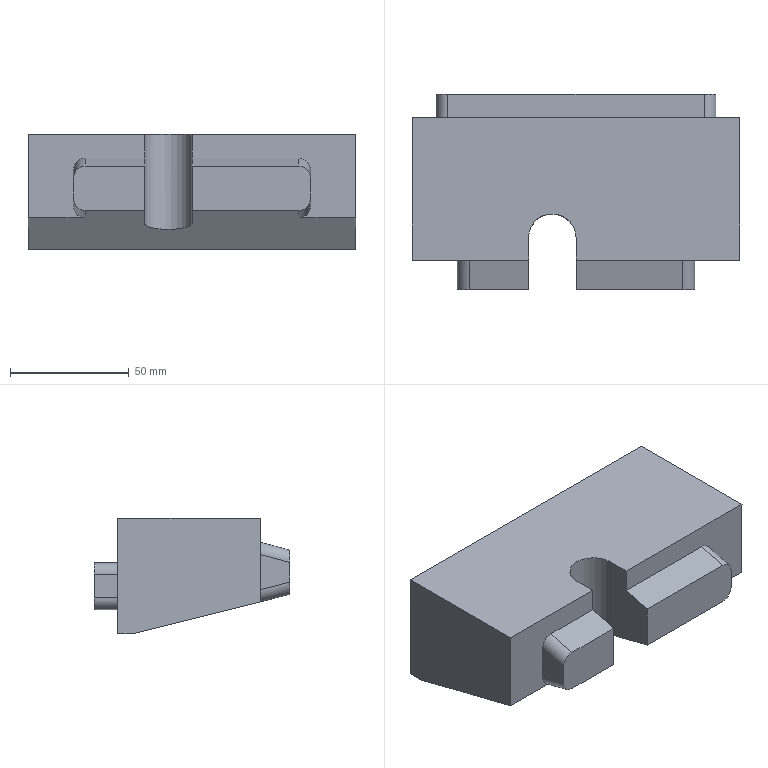Part | STEP file | WEDGE-2_id574_x_t | 1 solid | 30 faces | box 138 x 82.5 x 48.5 mm | volume 384224 mm3 | plane 21 | cylinder 9 | commonest cylinder face diameters 10 x8 20 x1
STEP:
#1=CARTESIAN_POINT('',(-79.,10.5,241.503));
#2=VERTEX_POINT('',#1);
#3=CARTESIAN_POINT('',(-79.,10.5,251.503));
#4=VERTEX_POINT('',#3);
#5=CARTESIAN_POINT('',(-79.,10.5,232.37));
#6=DIRECTION('',(0.,0.,1.));
#7=VECTOR('',#6,1.);
#8=LINE('',#5,#7);
#9=EDGE_CURVE('',#2,#4,#8,.T.);
#10=ORIENTED_EDGE('',*,*,#9,.T.);
#11=CARTESIAN_POINT('',(-74.,10.5,256.503));
#12=VERTEX_POINT('',#11);
#13=CARTESIAN_POINT('',(-74.,10.5,251.503));
#14=DIRECTION('',(0.,-1.,0.));
#15=DIRECTION('',(0.,0.,-1.));
#16=AXIS2_PLACEMENT_3D('',#13,#14,#15);
#17=CIRCLE('',#16,5.);
#18=EDGE_CURVE('',#12,#4,#17,.T.);
#19=ORIENTED_EDGE('',*,*,#18,.F.);
#20=CARTESIAN_POINT('',(34.,10.5,256.503));
#21=VERTEX_POINT('',#20);
#22=CARTESIAN_POINT('',(-89.,10.5,256.503));
#23=DIRECTION('',(-1.,0.,0.));
#24=VECTOR('',#23,1.);
#25=LINE('',#22,#24);
#26=EDGE_CURVE('',#21,#12,#25,.T.);
#27=ORIENTED_EDGE('',*,*,#26,.F.);
#28=CARTESIAN_POINT('',(39.,10.5,251.503));
#29=VERTEX_POINT('',#28);
#30=CARTESIAN_POINT('',(34.,10.5,251.503));
#31=DIRECTION('',(0.,-1.,0.));
#32=DIRECTION('',(0.,0.,1.));
#33=AXIS2_PLACEMENT_3D('',#30,#31,#32);
#34=CIRCLE('',#33,5.);
#35=EDGE_CURVE('',#29,#21,#34,.T.);
#36=ORIENTED_EDGE('',*,*,#35,.F.);
#37=CARTESIAN_POINT('',(39.,10.5,241.503));
#38=VERTEX_POINT('',#37);
#39=CARTESIAN_POINT('',(39.,10.5,260.794));
#40=DIRECTION('',(0.,0.,-1.));
#41=VECTOR('',#40,1.);
#42=LINE('',#39,#41);
#43=EDGE_CURVE('',#29,#38,#42,.T.);
#44=ORIENTED_EDGE('',*,*,#43,.T.);
#45=CARTESIAN_POINT('',(34.,10.5,236.503));
#46=VERTEX_POINT('',#45);
#47=CARTESIAN_POINT('',(34.,10.5,241.503));
#48=DIRECTION('',(0.,-1.,0.));
#49=DIRECTION('',(0.,0.,-1.));
#50=AXIS2_PLACEMENT_3D('',#47,#48,#49);
#51=CIRCLE('',#50,5.);
#52=EDGE_CURVE('',#46,#38,#51,.T.);
#53=ORIENTED_EDGE('',*,*,#52,.F.);
#54=CARTESIAN_POINT('',(-74.,10.5,236.503));
#55=VERTEX_POINT('',#54);
#56=CARTESIAN_POINT('',(-89.,10.5,236.503));
#57=DIRECTION('',(1.,0.,0.));
#58=VECTOR('',#57,1.);
#59=LINE('',#56,#58);
#60=EDGE_CURVE('',#55,#46,#59,.T.);
#61=ORIENTED_EDGE('',*,*,#60,.F.);
#62=CARTESIAN_POINT('',(-74.,10.5,241.503));
#63=DIRECTION('',(0.,-1.,0.));
#64=DIRECTION('',(0.,0.,1.));
#65=AXIS2_PLACEMENT_3D('',#62,#63,#64);
#66=CIRCLE('',#65,5.);
#67=EDGE_CURVE('',#2,#55,#66,.T.);
#68=ORIENTED_EDGE('',*,*,#67,.F.);
#69=EDGE_LOOP('',(#10,#19,#27,#36,#44,#53,#61,#68));
#70=FACE_OUTER_BOUND('',#69,.T.);
#71=CARTESIAN_POINT('',(-89.,10.5,236.503));
#72=DIRECTION('',(0.,1.,0.));
#73=DIRECTION('',(0.,0.,1.));
#74=AXIS2_PLACEMENT_3D('',#71,#72,#73);
#75=PLANE('',#74);
#76=ADVANCED_FACE('',(#70),#75,.T.);
#77=ORIENTED_EDGE('',*,*,#18,.T.);
#78=CARTESIAN_POINT('',(-79.,0.5,251.503));
#79=VERTEX_POINT('',#78);
#80=CARTESIAN_POINT('',(-79.,0.5,251.503));
#81=DIRECTION('',(0.,-1.,0.));
#82=VECTOR('',#81,1.);
#83=LINE('',#80,#82);
#84=EDGE_CURVE('',#4,#79,#83,.T.);
#85=ORIENTED_EDGE('',*,*,#84,.T.);
#86=CARTESIAN_POINT('',(-74.,0.5,256.503));
#87=VERTEX_POINT('',#86);
#88=CARTESIAN_POINT('',(-74.,0.5,251.503));
#89=DIRECTION('',(0.,-1.,0.));
#90=DIRECTION('',(0.,0.,-1.));
#91=AXIS2_PLACEMENT_3D('',#88,#89,#90);
#92=CIRCLE('',#91,5.);
#93=EDGE_CURVE('',#87,#79,#92,.T.);
#94=ORIENTED_EDGE('',*,*,#93,.F.);
#95=CARTESIAN_POINT('',(-74.,10.5,256.503));
#96=DIRECTION('',(0.,-1.,0.));
#97=VECTOR('',#96,1.);
#98=LINE('',#95,#97);
#99=EDGE_CURVE('',#12,#87,#98,.T.);
#100=ORIENTED_EDGE('',*,*,#99,.F.);
#101=EDGE_LOOP('',(#77,#85,#94,#100));
#102=FACE_OUTER_BOUND('',#101,.T.);
#103=CARTESIAN_POINT('',(-74.,10.725,251.503));
#104=DIRECTION('',(0.,-1.,0.));
#105=DIRECTION('',(0.,0.,-1.));
#106=AXIS2_PLACEMENT_3D('',#103,#104,#105);
#107=CYLINDRICAL_SURFACE('',#106,5.);
#108=ADVANCED_FACE('',(#102),#107,.T.);
#109=CARTESIAN_POINT('',(-79.,0.5,241.503));
#110=VERTEX_POINT('',#109);
#111=CARTESIAN_POINT('',(-79.,0.2283,241.503));
#112=DIRECTION('',(0.,1.,0.));
#113=VECTOR('',#112,1.);
#114=LINE('',#111,#113);
#115=EDGE_CURVE('',#110,#2,#114,.T.);
#116=ORIENTED_EDGE('',*,*,#115,.F.);
#117=CARTESIAN_POINT('',(-79.,0.5,226.503));
#118=DIRECTION('',(0.,0.,-1.));
#119=VECTOR('',#118,1.);
#120=LINE('',#117,#119);
#121=EDGE_CURVE('',#79,#110,#120,.T.);
#122=ORIENTED_EDGE('',*,*,#121,.F.);
#123=ORIENTED_EDGE('',*,*,#84,.F.);
#124=ORIENTED_EDGE('',*,*,#9,.F.);
#125=EDGE_LOOP('',(#116,#122,#123,#124));
#126=FACE_OUTER_BOUND('',#125,.T.);
#127=CARTESIAN_POINT('',(-79.,0.5,232.37));
#128=DIRECTION('',(1.,0.,0.));
#129=DIRECTION('',(0.,0.,-1.));
#130=AXIS2_PLACEMENT_3D('',#127,#128,#129);
#131=PLANE('',#130);
#132=ADVANCED_FACE('',(#126),#131,.F.);
#133=CARTESIAN_POINT('',(-74.,0.5,236.503));
#134=VERTEX_POINT('',#133);
#135=CARTESIAN_POINT('',(-74.,0.5,241.503));
#136=DIRECTION('',(0.,-1.,0.));
#137=DIRECTION('',(0.,0.,1.));
#138=AXIS2_PLACEMENT_3D('',#135,#136,#137);
#139=CIRCLE('',#138,5.);
#140=EDGE_CURVE('',#110,#134,#139,.T.);
#141=ORIENTED_EDGE('',*,*,#140,.F.);
#142=ORIENTED_EDGE('',*,*,#115,.T.);
#143=ORIENTED_EDGE('',*,*,#67,.T.);
#144=CARTESIAN_POINT('',(-74.,0.5,236.503));
#145=DIRECTION('',(0.,1.,0.));
#146=VECTOR('',#145,1.);
#147=LINE('',#144,#146);
#148=EDGE_CURVE('',#134,#55,#147,.T.);
#149=ORIENTED_EDGE('',*,*,#148,.F.);
#150=EDGE_LOOP('',(#141,#142,#143,#149));
#151=FACE_OUTER_BOUND('',#150,.T.);
#152=CARTESIAN_POINT('',(-74.,0.2283,241.503));
#153=DIRECTION('',(0.,1.,0.));
#154=DIRECTION('',(0.,0.,1.));
#155=AXIS2_PLACEMENT_3D('',#152,#153,#154);
#156=CYLINDRICAL_SURFACE('',#155,5.);
#157=ADVANCED_FACE('',(#151),#156,.T.);
#158=CARTESIAN_POINT('',(34.,0.5,236.503));
#159=VERTEX_POINT('',#158);
#160=CARTESIAN_POINT('',(-89.,0.5,236.503));
#161=DIRECTION('',(1.,0.,0.));
#162=VECTOR('',#161,1.);
#163=LINE('',#160,#162);
#164=EDGE_CURVE('',#134,#159,#163,.T.);
#165=ORIENTED_EDGE('',*,*,#164,.F.);
#166=ORIENTED_EDGE('',*,*,#148,.T.);
#167=ORIENTED_EDGE('',*,*,#60,.T.);
#168=CARTESIAN_POINT('',(34.,10.725,236.503));
#169=DIRECTION('',(0.,1.,0.));
#170=VECTOR('',#169,1.);
#171=LINE('',#168,#170);
#172=EDGE_CURVE('',#159,#46,#171,.T.);
#173=ORIENTED_EDGE('',*,*,#172,.F.);
#174=EDGE_LOOP('',(#165,#166,#167,#173));
#175=FACE_OUTER_BOUND('',#174,.T.);
#176=CARTESIAN_POINT('',(-89.,0.5,236.503));
#177=DIRECTION('',(0.,0.,-1.));
#178=DIRECTION('',(-1.,0.,0.));
#179=AXIS2_PLACEMENT_3D('',#176,#177,#178);
#180=PLANE('',#179);
#181=ADVANCED_FACE('',(#175),#180,.T.);
#182=ORIENTED_EDGE('',*,*,#52,.T.);
#183=CARTESIAN_POINT('',(39.,0.5,241.503));
#184=VERTEX_POINT('',#183);
#185=CARTESIAN_POINT('',(39.,0.5,241.503));
#186=DIRECTION('',(0.,-1.,0.));
#187=VECTOR('',#186,1.);
#188=LINE('',#185,#187);
#189=EDGE_CURVE('',#38,#184,#188,.T.);
#190=ORIENTED_EDGE('',*,*,#189,.T.);
#191=CARTESIAN_POINT('',(34.,0.5,241.503));
#192=DIRECTION('',(0.,-1.,0.));
#193=DIRECTION('',(0.,0.,-1.));
#194=AXIS2_PLACEMENT_3D('',#191,#192,#193);
#195=CIRCLE('',#194,5.);
#196=EDGE_CURVE('',#159,#184,#195,.T.);
#197=ORIENTED_EDGE('',*,*,#196,.F.);
#198=ORIENTED_EDGE('',*,*,#172,.T.);
#199=EDGE_LOOP('',(#182,#190,#197,#198));
#200=FACE_OUTER_BOUND('',#199,.T.);
#201=CARTESIAN_POINT('',(34.,10.725,241.503));
#202=DIRECTION('',(0.,-1.,0.));
#203=DIRECTION('',(0.,0.,-1.));
#204=AXIS2_PLACEMENT_3D('',#201,#202,#203);
#205=CYLINDRICAL_SURFACE('',#204,5.);
#206=ADVANCED_FACE('',(#200),#205,.T.);
#207=ORIENTED_EDGE('',*,*,#189,.F.);
#208=ORIENTED_EDGE('',*,*,#43,.F.);
#209=CARTESIAN_POINT('',(39.,0.5,251.503));
#210=VERTEX_POINT('',#209);
#211=CARTESIAN_POINT('',(39.,0.2508,251.503));
#212=DIRECTION('',(0.,1.,0.));
#213=VECTOR('',#212,1.);
#214=LINE('',#211,#213);
#215=EDGE_CURVE('',#210,#29,#214,.T.);
#216=ORIENTED_EDGE('',*,*,#215,.F.);
#217=CARTESIAN_POINT('',(39.,0.5,226.503));
#218=DIRECTION('',(0.,0.,1.));
#219=VECTOR('',#218,1.);
#220=LINE('',#217,#219);
#221=EDGE_CURVE('',#184,#210,#220,.T.);
#222=ORIENTED_EDGE('',*,*,#221,.F.);
#223=EDGE_LOOP('',(#207,#208,#216,#222));
#224=FACE_OUTER_BOUND('',#223,.T.);
#225=CARTESIAN_POINT('',(39.,0.5,260.794));
#226=DIRECTION('',(-1.,0.,0.));
#227=DIRECTION('',(0.,0.,1.));
#228=AXIS2_PLACEMENT_3D('',#225,#226,#227);
#229=PLANE('',#228);
#230=ADVANCED_FACE('',(#224),#229,.F.);
#231=CARTESIAN_POINT('',(34.,0.5,256.503));
#232=VERTEX_POINT('',#231);
#233=CARTESIAN_POINT('',(34.,0.5,251.503));
#234=DIRECTION('',(0.,-1.,0.));
#235=DIRECTION('',(0.,0.,1.));
#236=AXIS2_PLACEMENT_3D('',#233,#234,#235);
#237=CIRCLE('',#236,5.);
#238=EDGE_CURVE('',#210,#232,#237,.T.);
#239=ORIENTED_EDGE('',*,*,#238,.F.);
#240=ORIENTED_EDGE('',*,*,#215,.T.);
#241=ORIENTED_EDGE('',*,*,#35,.T.);
#242=CARTESIAN_POINT('',(34.,10.5,256.503));
#243=DIRECTION('',(0.,1.,0.));
#244=VECTOR('',#243,1.);
#245=LINE('',#242,#244);
#246=EDGE_CURVE('',#232,#21,#245,.T.);
#247=ORIENTED_EDGE('',*,*,#246,.F.);
#248=EDGE_LOOP('',(#239,#240,#241,#247));
#249=FACE_OUTER_BOUND('',#248,.T.);
#250=CARTESIAN_POINT('',(34.,0.2508,251.503));
#251=DIRECTION('',(0.,1.,0.));
#252=DIRECTION('',(0.,0.,1.));
#253=AXIS2_PLACEMENT_3D('',#250,#251,#252);
#254=CYLINDRICAL_SURFACE('',#253,5.);
#255=ADVANCED_FACE('',(#249),#254,.T.);
#256=ORIENTED_EDGE('',*,*,#26,.T.);
#257=ORIENTED_EDGE('',*,*,#99,.T.);
#258=CARTESIAN_POINT('',(-89.,0.5,256.503));
#259=DIRECTION('',(-1.,0.,0.));
#260=VECTOR('',#259,1.);
#261=LINE('',#258,#260);
#262=EDGE_CURVE('',#232,#87,#261,.T.);
#263=ORIENTED_EDGE('',*,*,#262,.F.);
#264=ORIENTED_EDGE('',*,*,#246,.T.);
#265=EDGE_LOOP('',(#256,#257,#263,#264));
#266=FACE_OUTER_BOUND('',#265,.T.);
#267=CARTESIAN_POINT('',(-89.,10.5,256.503));
#268=DIRECTION('',(0.,0.,1.));
#269=DIRECTION('',(1.,0.,0.));
#270=AXIS2_PLACEMENT_3D('',#267,#268,#269);
#271=PLANE('',#270);
#272=ADVANCED_FACE('',(#266),#271,.T.);
#273=CARTESIAN_POINT('',(-70.,-59.5,259.826));
#274=VERTEX_POINT('',#273);
#275=CARTESIAN_POINT('',(-70.,-72.,256.477));
#276=VERTEX_POINT('',#275);
#277=CARTESIAN_POINT('',(-70.,-57.911,260.252));
#278=DIRECTION('',(0.,-0.9659,-0.2588));
#279=VECTOR('',#278,1.);
#280=LINE('',#277,#279);
#281=EDGE_CURVE('',#274,#276,#280,.T.);
#282=ORIENTED_EDGE('',*,*,#281,.F.);
#283=CARTESIAN_POINT('',(-70.,-59.5,245.018));
#284=VERTEX_POINT('',#283);
#285=CARTESIAN_POINT('',(-70.,-59.5,275.003));
#286=DIRECTION('',(0.,0.,1.));
#287=VECTOR('',#286,1.);
#288=LINE('',#285,#287);
#289=EDGE_CURVE('',#284,#274,#288,.T.);
#290=ORIENTED_EDGE('',*,*,#289,.F.);
#291=CARTESIAN_POINT('',(-70.,-72.,248.134));
#292=VERTEX_POINT('',#291);
#293=CARTESIAN_POINT('',(-70.,-72.472,248.252));
#294=DIRECTION('',(0.,0.9703,-0.2419));
#295=VECTOR('',#294,1.);
#296=LINE('',#293,#295);
#297=EDGE_CURVE('',#292,#284,#296,.T.);
#298=ORIENTED_EDGE('',*,*,#297,.F.);
#299=CARTESIAN_POINT('',(-70.,-72.,261.654));
#300=DIRECTION('',(0.,0.,-1.));
#301=VECTOR('',#300,1.);
#302=LINE('',#299,#301);
#303=EDGE_CURVE('',#276,#292,#302,.T.);
#304=ORIENTED_EDGE('',*,*,#303,.F.);
#305=EDGE_LOOP('',(#282,#290,#298,#304));
#306=FACE_OUTER_BOUND('',#305,.T.);
#307=CARTESIAN_POINT('',(-70.,-59.5,226.503));
#308=DIRECTION('',(1.,0.,0.));
#309=DIRECTION('',(0.,0.,-1.));
#310=AXIS2_PLACEMENT_3D('',#307,#308,#309);
#311=PLANE('',#310);
#312=ADVANCED_FACE('',(#306),#311,.F.);
#313=CARTESIAN_POINT('',(-65.,-59.5,265.003));
#314=VERTEX_POINT('',#313);
#315=CARTESIAN_POINT('',(-65.,-59.5,259.826));
#316=DIRECTION('',(0.,1.,0.));
#317=DIRECTION('',(0.,0.,-1.));
#318=AXIS2_PLACEMENT_3D('',#315,#316,#317);
#319=ELLIPSE('',#318,5.176,5.);
#320=EDGE_CURVE('',#274,#314,#319,.T.);
#321=ORIENTED_EDGE('',*,*,#320,.F.);
#322=ORIENTED_EDGE('',*,*,#281,.T.);
#323=CARTESIAN_POINT('',(-65.,-72.,261.654));
#324=VERTEX_POINT('',#323);
#325=CARTESIAN_POINT('',(-65.,-72.,256.477));
#326=DIRECTION('',(0.,-1.,0.));
#327=DIRECTION('',(0.,0.,-1.));
#328=AXIS2_PLACEMENT_3D('',#325,#326,#327);
#329=ELLIPSE('',#328,5.176,5.);
#330=EDGE_CURVE('',#324,#276,#329,.T.);
#331=ORIENTED_EDGE('',*,*,#330,.F.);
#332=CARTESIAN_POINT('',(-65.,-59.5,265.003));
#333=DIRECTION('',(0.,-0.9659,-0.2588));
#334=VECTOR('',#333,1.);
#335=LINE('',#332,#334);
#336=EDGE_CURVE('',#314,#324,#335,.T.);
#337=ORIENTED_EDGE('',*,*,#336,.F.);
#338=EDGE_LOOP('',(#321,#322,#331,#337));
#339=FACE_OUTER_BOUND('',#338,.T.);
#340=CARTESIAN_POINT('',(-65.,-57.911,260.252));
#341=DIRECTION('',(0.,-0.9659,-0.2588));
#342=DIRECTION('',(0.,0.2588,-0.9659));
#343=AXIS2_PLACEMENT_3D('',#340,#341,#342);
#344=CYLINDRICAL_SURFACE('',#343,5.);
#345=ADVANCED_FACE('',(#339),#344,.T.);
#346=CARTESIAN_POINT('',(-40.,-72.,261.654));
#347=VERTEX_POINT('',#346);
#348=CARTESIAN_POINT('',(-89.,-72.,261.654));
#349=DIRECTION('',(-1.,0.,0.));
#350=VECTOR('',#349,1.);
#351=LINE('',#348,#350);
#352=EDGE_CURVE('',#347,#324,#351,.T.);
#353=ORIENTED_EDGE('',*,*,#352,.F.);
#354=CARTESIAN_POINT('',(-40.,-59.5,265.003));
#355=VERTEX_POINT('',#354);
#356=CARTESIAN_POINT('',(-40.,-72.,261.654));
#357=DIRECTION('',(0.,0.9659,0.2588));
#358=VECTOR('',#357,1.);
#359=LINE('',#356,#358);
#360=EDGE_CURVE('',#347,#355,#359,.T.);
#361=ORIENTED_EDGE('',*,*,#360,.T.);
#362=CARTESIAN_POINT('',(-89.,-59.5,265.003));
#363=DIRECTION('',(1.,0.,0.));
#364=VECTOR('',#363,1.);
#365=LINE('',#362,#364);
#366=EDGE_CURVE('',#314,#355,#365,.T.);
#367=ORIENTED_EDGE('',*,*,#366,.F.);
#368=ORIENTED_EDGE('',*,*,#336,.T.);
#369=EDGE_LOOP('',(#353,#361,#367,#368));
#370=FACE_OUTER_BOUND('',#369,.T.);
#371=CARTESIAN_POINT('',(-89.,-59.5,265.003));
#372=DIRECTION('',(0.,-0.2588,0.9659));
#373=DIRECTION('',(0.,-0.9659,-0.2588));
#374=AXIS2_PLACEMENT_3D('',#371,#372,#373);
#375=PLANE('',#374);
#376=ADVANCED_FACE('',(#370),#375,.T.);
#377=ORIENTED_EDGE('',*,*,#238,.T.);
#378=ORIENTED_EDGE('',*,*,#262,.T.);
#379=ORIENTED_EDGE('',*,*,#93,.T.);
#380=ORIENTED_EDGE('',*,*,#121,.T.);
#381=ORIENTED_EDGE('',*,*,#140,.T.);
#382=ORIENTED_EDGE('',*,*,#164,.T.);
#383=ORIENTED_EDGE('',*,*,#196,.T.);
#384=ORIENTED_EDGE('',*,*,#221,.T.);
#385=EDGE_LOOP('',(#377,#378,#379,#380,#381,#382,#383,#384));
#386=FACE_BOUND('',#385,.T.);
#387=CARTESIAN_POINT('',(49.,0.5,275.003));
#388=VERTEX_POINT('',#387);
#389=CARTESIAN_POINT('',(-89.,0.5,275.003));
#390=VERTEX_POINT('',#389);
#391=CARTESIAN_POINT('',(-89.,0.5,275.003));
#392=DIRECTION('',(-1.,0.,0.));
#393=VECTOR('',#392,1.);
#394=LINE('',#391,#393);
#395=EDGE_CURVE('',#388,#390,#394,.T.);
#396=ORIENTED_EDGE('',*,*,#395,.F.);
#397=CARTESIAN_POINT('',(49.,0.5,226.503));
#398=VERTEX_POINT('',#397);
#399=CARTESIAN_POINT('',(49.,0.5,160.003));
#400=DIRECTION('',(0.,0.,1.));
#401=VECTOR('',#400,1.);
#402=LINE('',#399,#401);
#403=EDGE_CURVE('',#398,#388,#402,.T.);
#404=ORIENTED_EDGE('',*,*,#403,.F.);
#405=CARTESIAN_POINT('',(-89.,0.5,226.503));
#406=VERTEX_POINT('',#405);
#407=CARTESIAN_POINT('',(-89.,0.5,226.503));
#408=DIRECTION('',(1.,0.,0.));
#409=VECTOR('',#408,1.);
#410=LINE('',#407,#409);
#411=EDGE_CURVE('',#406,#398,#410,.T.);
#412=ORIENTED_EDGE('',*,*,#411,.F.);
#413=CARTESIAN_POINT('',(-89.,0.5,160.003));
#414=DIRECTION('',(0.,0.,1.));
#415=VECTOR('',#414,1.);
#416=LINE('',#413,#415);
#417=EDGE_CURVE('',#406,#390,#416,.T.);
#418=ORIENTED_EDGE('',*,*,#417,.T.);
#419=EDGE_LOOP('',(#396,#404,#412,#418));
#420=FACE_BOUND('',#419,.T.);
#421=CARTESIAN_POINT('',(-89.,0.5,226.503));
#422=DIRECTION('',(0.,1.,0.));
#423=DIRECTION('',(0.,0.,1.));
#424=AXIS2_PLACEMENT_3D('',#421,#422,#423);
#425=PLANE('',#424);
#426=ADVANCED_FACE('',(#386,#420),#425,.T.);
#427=CARTESIAN_POINT('',(30.,-72.,256.477));
#428=VERTEX_POINT('',#427);
#429=CARTESIAN_POINT('',(30.,-59.5,259.826));
#430=VERTEX_POINT('',#429);
#431=CARTESIAN_POINT('',(30.,-72.414,256.366));
#432=DIRECTION('',(0.,0.9659,0.2588));
#433=VECTOR('',#432,1.);
#434=LINE('',#431,#433);
#435=EDGE_CURVE('',#428,#430,#434,.T.);
#436=ORIENTED_EDGE('',*,*,#435,.F.);
#437=CARTESIAN_POINT('',(30.,-72.,248.134));
#438=VERTEX_POINT('',#437);
#439=CARTESIAN_POINT('',(30.,-72.,261.654));
#440=DIRECTION('',(0.,0.,1.));
#441=VECTOR('',#440,1.);
#442=LINE('',#439,#441);
#443=EDGE_CURVE('',#438,#428,#442,.T.);
#444=ORIENTED_EDGE('',*,*,#443,.F.);
#445=CARTESIAN_POINT('',(30.,-59.5,245.018));
#446=VERTEX_POINT('',#445);
#447=CARTESIAN_POINT('',(30.,-4.303,231.256));
#448=DIRECTION('',(0.,-0.9703,0.2419));
#449=VECTOR('',#448,1.);
#450=LINE('',#447,#449);
#451=EDGE_CURVE('',#446,#438,#450,.T.);
#452=ORIENTED_EDGE('',*,*,#451,.F.);
#453=CARTESIAN_POINT('',(30.,-59.5,275.003));
#454=DIRECTION('',(0.,0.,-1.));
#455=VECTOR('',#454,1.);
#456=LINE('',#453,#455);
#457=EDGE_CURVE('',#430,#446,#456,.T.);
#458=ORIENTED_EDGE('',*,*,#457,.F.);
#459=EDGE_LOOP('',(#436,#444,#452,#458));
#460=FACE_OUTER_BOUND('',#459,.T.);
#461=CARTESIAN_POINT('',(30.,-59.5,275.003));
#462=DIRECTION('',(-1.,0.,0.));
#463=DIRECTION('',(0.,0.,1.));
#464=AXIS2_PLACEMENT_3D('',#461,#462,#463);
#465=PLANE('',#464);
#466=ADVANCED_FACE('',(#460),#465,.F.);
#467=CARTESIAN_POINT('',(25.,-72.,261.654));
#468=VERTEX_POINT('',#467);
#469=CARTESIAN_POINT('',(25.,-72.,256.477));
#470=DIRECTION('',(0.,-1.,0.));
#471=DIRECTION('',(0.,0.,1.));
#472=AXIS2_PLACEMENT_3D('',#469,#470,#471);
#473=ELLIPSE('',#472,5.176,5.);
#474=EDGE_CURVE('',#428,#468,#473,.T.);
#475=ORIENTED_EDGE('',*,*,#474,.F.);
#476=ORIENTED_EDGE('',*,*,#435,.T.);
#477=CARTESIAN_POINT('',(25.,-59.5,265.003));
#478=VERTEX_POINT('',#477);
#479=CARTESIAN_POINT('',(25.,-59.5,259.826));
#480=DIRECTION('',(0.,1.,0.));
#481=DIRECTION('',(0.,0.,1.));
#482=AXIS2_PLACEMENT_3D('',#479,#480,#481);
#483=ELLIPSE('',#482,5.176,5.);
#484=EDGE_CURVE('',#478,#430,#483,.T.);
#485=ORIENTED_EDGE('',*,*,#484,.F.);
#486=CARTESIAN_POINT('',(25.,-59.5,265.003));
#487=DIRECTION('',(0.,0.9659,0.2588));
#488=VECTOR('',#487,1.);
#489=LINE('',#486,#488);
#490=EDGE_CURVE('',#468,#478,#489,.T.);
#491=ORIENTED_EDGE('',*,*,#490,.F.);
#492=EDGE_LOOP('',(#475,#476,#485,#491));
#493=FACE_OUTER_BOUND('',#492,.T.);
#494=CARTESIAN_POINT('',(25.,-72.414,256.366));
#495=DIRECTION('',(0.,0.9659,0.2588));
#496=DIRECTION('',(0.,-0.2588,0.9659));
#497=AXIS2_PLACEMENT_3D('',#494,#495,#496);
#498=CYLINDRICAL_SURFACE('',#497,5.);
#499=ADVANCED_FACE('',(#493),#498,.T.);
#500=CARTESIAN_POINT('',(-20.,-59.5,265.003));
#501=VERTEX_POINT('',#500);
#502=CARTESIAN_POINT('',(-89.,-59.5,265.003));
#503=DIRECTION('',(1.,0.,0.));
#504=VECTOR('',#503,1.);
#505=LINE('',#502,#504);
#506=EDGE_CURVE('',#501,#478,#505,.T.);
#507=ORIENTED_EDGE('',*,*,#506,.F.);
#508=CARTESIAN_POINT('',(-20.,-72.,261.654));
#509=VERTEX_POINT('',#508);
#510=CARTESIAN_POINT('',(-20.,-59.5,265.003));
#511=DIRECTION('',(0.,-0.9659,-0.2588));
#512=VECTOR('',#511,1.);
#513=LINE('',#510,#512);
#514=EDGE_CURVE('',#501,#509,#513,.T.);
#515=ORIENTED_EDGE('',*,*,#514,.T.);
#516=CARTESIAN_POINT('',(-89.,-72.,261.654));
#517=DIRECTION('',(-1.,0.,0.));
#518=VECTOR('',#517,1.);
#519=LINE('',#516,#518);
#520=EDGE_CURVE('',#468,#509,#519,.T.);
#521=ORIENTED_EDGE('',*,*,#520,.F.);
#522=ORIENTED_EDGE('',*,*,#490,.T.);
#523=EDGE_LOOP('',(#507,#515,#521,#522));
#524=FACE_OUTER_BOUND('',#523,.T.);
#525=CARTESIAN_POINT('',(-89.,-59.5,265.003));
#526=DIRECTION('',(0.,-0.2588,0.9659));
#527=DIRECTION('',(0.,-0.9659,-0.2588));
#528=AXIS2_PLACEMENT_3D('',#525,#526,#527);
#529=PLANE('',#528);
#530=ADVANCED_FACE('',(#524),#529,.T.);
#531=CARTESIAN_POINT('',(-40.,-59.5,275.003));
#532=VERTEX_POINT('',#531);
#533=CARTESIAN_POINT('',(-40.,-50.,275.003));
#534=VERTEX_POINT('',#533);
#535=CARTESIAN_POINT('',(-40.,-72.,275.003));
#536=DIRECTION('',(0.,1.,0.));
#537=VECTOR('',#536,1.);
#538=LINE('',#535,#537);
#539=EDGE_CURVE('',#532,#534,#538,.T.);
#540=ORIENTED_EDGE('',*,*,#539,.T.);
#541=CARTESIAN_POINT('',(-20.,-50.,275.003));
#542=VERTEX_POINT('',#541);
#543=CARTESIAN_POINT('',(-30.,-50.,275.003));
#544=DIRECTION('',(0.,0.,-1.));
#545=DIRECTION('',(-1.,0.,0.));
#546=AXIS2_PLACEMENT_3D('',#543,#544,#545);
#547=CIRCLE('',#546,10.);
#548=EDGE_CURVE('',#534,#542,#547,.T.);
#549=ORIENTED_EDGE('',*,*,#548,.T.);
#550=CARTESIAN_POINT('',(-20.,-59.5,275.003));
#551=VERTEX_POINT('',#550);
#552=CARTESIAN_POINT('',(-20.,-50.,275.003));
#553=DIRECTION('',(0.,-1.,0.));
#554=VECTOR('',#553,1.);
#555=LINE('',#552,#554);
#556=EDGE_CURVE('',#542,#551,#555,.T.);
#557=ORIENTED_EDGE('',*,*,#556,.T.);
#558=CARTESIAN_POINT('',(49.,-59.5,275.003));
#559=VERTEX_POINT('',#558);
#560=CARTESIAN_POINT('',(-89.,-59.5,275.003));
#561=DIRECTION('',(-1.,0.,0.));
#562=VECTOR('',#561,1.);
#563=LINE('',#560,#562);
#564=EDGE_CURVE('',#559,#551,#563,.T.);
#565=ORIENTED_EDGE('',*,*,#564,.F.);
#566=CARTESIAN_POINT('',(49.,0.,275.003));
#567=DIRECTION('',(0.,-1.,0.));
#568=VECTOR('',#567,1.);
#569=LINE('',#566,#568);
#570=EDGE_CURVE('',#388,#559,#569,.T.);
#571=ORIENTED_EDGE('',*,*,#570,.F.);
#572=ORIENTED_EDGE('',*,*,#395,.T.);
#573=CARTESIAN_POINT('',(-89.,-59.5,275.003));
#574=VERTEX_POINT('',#573);
#575=CARTESIAN_POINT('',(-89.,0.,275.003));
#576=DIRECTION('',(0.,-1.,0.));
#577=VECTOR('',#576,1.);
#578=LINE('',#575,#577);
#579=EDGE_CURVE('',#390,#574,#578,.T.);
#580=ORIENTED_EDGE('',*,*,#579,.T.);
#581=CARTESIAN_POINT('',(-89.,-59.5,275.003));
#582=DIRECTION('',(-1.,0.,0.));
#583=VECTOR('',#582,1.);
#584=LINE('',#581,#583);
#585=EDGE_CURVE('',#532,#574,#584,.T.);
#586=ORIENTED_EDGE('',*,*,#585,.F.);
#587=EDGE_LOOP('',(#540,#549,#557,#565,#571,#572,#580,#586));
#588=FACE_OUTER_BOUND('',#587,.T.);
#589=CARTESIAN_POINT('',(-89.,0.5,275.003));
#590=DIRECTION('',(0.,0.,1.));
#591=DIRECTION('',(1.,0.,0.));
#592=AXIS2_PLACEMENT_3D('',#589,#590,#591);
#593=PLANE('',#592);
#594=ADVANCED_FACE('',(#588),#593,.T.);
#595=ORIENTED_EDGE('',*,*,#360,.F.);
#596=CARTESIAN_POINT('',(-40.,-72.,242.981));
#597=VERTEX_POINT('',#596);
#598=CARTESIAN_POINT('',(-40.,-72.,261.654));
#599=DIRECTION('',(0.,0.,1.));
#600=VECTOR('',#599,1.);
#601=LINE('',#598,#600);
#602=EDGE_CURVE('',#597,#347,#601,.T.);
#603=ORIENTED_EDGE('',*,*,#602,.F.);
#604=CARTESIAN_POINT('',(-40.,-50.,237.496));
#605=VERTEX_POINT('',#604);
#606=CARTESIAN_POINT('',(-40.,-72.,242.981));
#607=DIRECTION('',(0.,-0.9703,0.2419));
#608=VECTOR('',#607,1.);
#609=LINE('',#606,#608);
#610=EDGE_CURVE('',#605,#597,#609,.T.);
#611=ORIENTED_EDGE('',*,*,#610,.F.);
#612=CARTESIAN_POINT('',(-40.,-50.,226.503));
#613=DIRECTION('',(0.,0.,1.));
#614=VECTOR('',#613,1.);
#615=LINE('',#612,#614);
#616=EDGE_CURVE('',#605,#534,#615,.T.);
#617=ORIENTED_EDGE('',*,*,#616,.T.);
#618=ORIENTED_EDGE('',*,*,#539,.F.);
#619=CARTESIAN_POINT('',(-40.,-59.5,275.003));
#620=DIRECTION('',(0.,0.,1.));
#621=VECTOR('',#620,1.);
#622=LINE('',#619,#621);
#623=EDGE_CURVE('',#355,#532,#622,.T.);
#624=ORIENTED_EDGE('',*,*,#623,.F.);
#625=EDGE_LOOP('',(#595,#603,#611,#617,#618,#624));
#626=FACE_OUTER_BOUND('',#625,.T.);
#627=CARTESIAN_POINT('',(-40.,-72.,226.503));
#628=DIRECTION('',(-1.,0.,0.));
#629=DIRECTION('',(0.,0.,1.));
#630=AXIS2_PLACEMENT_3D('',#627,#628,#629);
#631=PLANE('',#630);
#632=ADVANCED_FACE('',(#626),#631,.F.);
#633=CARTESIAN_POINT('',(-65.,-72.,242.981));
#634=VERTEX_POINT('',#633);
#635=CARTESIAN_POINT('',(-89.,-72.,242.981));
#636=DIRECTION('',(-1.,0.,0.));
#637=VECTOR('',#636,1.);
#638=LINE('',#635,#637);
#639=EDGE_CURVE('',#597,#634,#638,.T.);
#640=ORIENTED_EDGE('',*,*,#639,.F.);
#641=ORIENTED_EDGE('',*,*,#602,.T.);
#642=ORIENTED_EDGE('',*,*,#352,.T.);
#643=ORIENTED_EDGE('',*,*,#330,.T.);
#644=ORIENTED_EDGE('',*,*,#303,.T.);
#645=CARTESIAN_POINT('',(-65.,-72.,248.134));
#646=DIRECTION('',(0.,1.,0.));
#647=DIRECTION('',(0.,0.,-1.));
#648=AXIS2_PLACEMENT_3D('',#645,#646,#647);
#649=ELLIPSE('',#648,5.153,5.);
#650=EDGE_CURVE('',#634,#292,#649,.T.);
#651=ORIENTED_EDGE('',*,*,#650,.F.);
#652=EDGE_LOOP('',(#640,#641,#642,#643,#644,#651));
#653=FACE_OUTER_BOUND('',#652,.T.);
#654=CARTESIAN_POINT('',(-89.,-72.,261.654));
#655=DIRECTION('',(0.,-1.,0.));
#656=DIRECTION('',(0.,0.,-1.));
#657=AXIS2_PLACEMENT_3D('',#654,#655,#656);
#658=PLANE('',#657);
#659=ADVANCED_FACE('',(#653),#658,.T.);
#660=ORIENTED_EDGE('',*,*,#650,.T.);
#661=ORIENTED_EDGE('',*,*,#297,.T.);
#662=CARTESIAN_POINT('',(-65.,-59.5,239.865));
#663=VERTEX_POINT('',#662);
#664=CARTESIAN_POINT('',(-65.,-59.5,245.018));
#665=DIRECTION('',(0.,1.,0.));
#666=DIRECTION('',(0.,0.,-1.));
#667=AXIS2_PLACEMENT_3D('',#664,#665,#666);
#668=ELLIPSE('',#667,5.153,5.);
#669=EDGE_CURVE('',#663,#284,#668,.T.);
#670=ORIENTED_EDGE('',*,*,#669,.F.);
#671=CARTESIAN_POINT('',(-65.,-72.,242.981));
#672=DIRECTION('',(0.,0.9703,-0.2419));
#673=VECTOR('',#672,1.);
#674=LINE('',#671,#673);
#675=EDGE_CURVE('',#634,#663,#674,.T.);
#676=ORIENTED_EDGE('',*,*,#675,.F.);
#677=EDGE_LOOP('',(#660,#661,#670,#676));
#678=FACE_OUTER_BOUND('',#677,.T.);
#679=CARTESIAN_POINT('',(-65.,-72.472,248.252));
#680=DIRECTION('',(0.,0.9703,-0.2419));
#681=DIRECTION('',(0.,0.2419,0.9703));
#682=AXIS2_PLACEMENT_3D('',#679,#680,#681);
#683=CYLINDRICAL_SURFACE('',#682,5.);
#684=ADVANCED_FACE('',(#678),#683,.T.);
#685=ORIENTED_EDGE('',*,*,#366,.T.);
#686=ORIENTED_EDGE('',*,*,#623,.T.);
#687=ORIENTED_EDGE('',*,*,#585,.T.);
#688=CARTESIAN_POINT('',(-89.,-59.5,239.865));
#689=VERTEX_POINT('',#688);
#690=CARTESIAN_POINT('',(-89.,-59.5,160.003));
#691=DIRECTION('',(0.,0.,-1.));
#692=VECTOR('',#691,1.);
#693=LINE('',#690,#692);
#694=EDGE_CURVE('',#574,#689,#693,.T.);
#695=ORIENTED_EDGE('',*,*,#694,.T.);
#696=CARTESIAN_POINT('',(-89.,-59.5,239.865));
#697=DIRECTION('',(-1.,0.,0.));
#698=VECTOR('',#697,1.);
#699=LINE('',#696,#698);
#700=EDGE_CURVE('',#663,#689,#699,.T.);
#701=ORIENTED_EDGE('',*,*,#700,.F.);
#702=ORIENTED_EDGE('',*,*,#669,.T.);
#703=ORIENTED_EDGE('',*,*,#289,.T.);
#704=ORIENTED_EDGE('',*,*,#320,.T.);
#705=EDGE_LOOP('',(#685,#686,#687,#695,#701,#702,#703,#704));
#706=FACE_OUTER_BOUND('',#705,.T.);
#707=CARTESIAN_POINT('',(-89.,-59.5,275.003));
#708=DIRECTION('',(0.,-1.,0.));
#709=DIRECTION('',(0.,0.,-1.));
#710=AXIS2_PLACEMENT_3D('',#707,#708,#709);
#711=PLANE('',#710);
#712=ADVANCED_FACE('',(#706),#711,.T.);
#713=CARTESIAN_POINT('',(-89.,-5.908,226.503));
#714=VERTEX_POINT('',#713);
#715=CARTESIAN_POINT('',(-89.,-72.,242.981));
#716=DIRECTION('',(0.,0.9703,-0.2419));
#717=VECTOR('',#716,1.);
#718=LINE('',#715,#717);
#719=EDGE_CURVE('',#689,#714,#718,.T.);
#720=ORIENTED_EDGE('',*,*,#719,.F.);
#721=ORIENTED_EDGE('',*,*,#694,.F.);
#722=ORIENTED_EDGE('',*,*,#579,.F.);
#723=ORIENTED_EDGE('',*,*,#417,.F.);
#724=CARTESIAN_POINT('',(-89.,-5.908,226.503));
#725=DIRECTION('',(0.,1.,0.));
#726=VECTOR('',#725,1.);
#727=LINE('',#724,#726);
#728=EDGE_CURVE('',#714,#406,#727,.T.);
#729=ORIENTED_EDGE('',*,*,#728,.F.);
#730=EDGE_LOOP('',(#720,#721,#722,#723,#729));
#731=FACE_OUTER_BOUND('',#730,.T.);
#732=CARTESIAN_POINT('',(-89.,0.,160.003));
#733=DIRECTION('',(1.,0.,0.));
#734=DIRECTION('',(0.,0.,-1.));
#735=AXIS2_PLACEMENT_3D('',#732,#733,#734);
#736=PLANE('',#735);
#737=ADVANCED_FACE('',(#731),#736,.F.);
#738=CARTESIAN_POINT('',(49.,-5.908,226.503));
#739=VERTEX_POINT('',#738);
#740=CARTESIAN_POINT('',(-89.,-5.908,226.503));
#741=DIRECTION('',(1.,0.,0.));
#742=VECTOR('',#741,1.);
#743=LINE('',#740,#742);
#744=EDGE_CURVE('',#714,#739,#743,.T.);
#745=ORIENTED_EDGE('',*,*,#744,.F.);
#746=ORIENTED_EDGE('',*,*,#728,.T.);
#747=ORIENTED_EDGE('',*,*,#411,.T.);
#748=CARTESIAN_POINT('',(49.,0.,226.503));
#749=DIRECTION('',(0.,1.,0.));
#750=VECTOR('',#749,1.);
#751=LINE('',#748,#750);
#752=EDGE_CURVE('',#739,#398,#751,.T.);
#753=ORIENTED_EDGE('',*,*,#752,.F.);
#754=EDGE_LOOP('',(#745,#746,#747,#753));
#755=FACE_OUTER_BOUND('',#754,.T.);
#756=CARTESIAN_POINT('',(-89.,-5.908,226.503));
#757=DIRECTION('',(0.,0.,-1.));
#758=DIRECTION('',(-1.,0.,0.));
#759=AXIS2_PLACEMENT_3D('',#756,#757,#758);
#760=PLANE('',#759);
#761=ADVANCED_FACE('',(#755),#760,.T.);
#762=ORIENTED_EDGE('',*,*,#752,.T.);
#763=ORIENTED_EDGE('',*,*,#403,.T.);
#764=ORIENTED_EDGE('',*,*,#570,.T.);
#765=CARTESIAN_POINT('',(49.,-59.5,239.865));
#766=VERTEX_POINT('',#765);
#767=CARTESIAN_POINT('',(49.,-59.5,275.003));
#768=DIRECTION('',(0.,0.,1.));
#769=VECTOR('',#768,1.);
#770=LINE('',#767,#769);
#771=EDGE_CURVE('',#766,#559,#770,.T.);
#772=ORIENTED_EDGE('',*,*,#771,.F.);
#773=CARTESIAN_POINT('',(49.,-72.,242.981));
#774=DIRECTION('',(0.,-0.9703,0.2419));
#775=VECTOR('',#774,1.);
#776=LINE('',#773,#775);
#777=EDGE_CURVE('',#739,#766,#776,.T.);
#778=ORIENTED_EDGE('',*,*,#777,.F.);
#779=EDGE_LOOP('',(#762,#763,#764,#772,#778));
#780=FACE_OUTER_BOUND('',#779,.T.);
#781=CARTESIAN_POINT('',(49.,0.,160.003));
#782=DIRECTION('',(1.,0.,0.));
#783=DIRECTION('',(0.,0.,-1.));
#784=AXIS2_PLACEMENT_3D('',#781,#782,#783);
#785=PLANE('',#784);
#786=ADVANCED_FACE('',(#780),#785,.T.);
#787=ORIENTED_EDGE('',*,*,#564,.T.);
#788=CARTESIAN_POINT('',(-20.,-59.5,226.503));
#789=DIRECTION('',(0.,0.,-1.));
#790=VECTOR('',#789,1.);
#791=LINE('',#788,#790);
#792=EDGE_CURVE('',#551,#501,#791,.T.);
#793=ORIENTED_EDGE('',*,*,#792,.T.);
#794=ORIENTED_EDGE('',*,*,#506,.T.);
#795=ORIENTED_EDGE('',*,*,#484,.T.);
#796=ORIENTED_EDGE('',*,*,#457,.T.);
#797=CARTESIAN_POINT('',(25.,-59.5,239.865));
#798=VERTEX_POINT('',#797);
#799=CARTESIAN_POINT('',(25.,-59.5,245.018));
#800=DIRECTION('',(0.,-1.,0.));
#801=DIRECTION('',(0.,0.,1.));
#802=AXIS2_PLACEMENT_3D('',#799,#800,#801);
#803=ELLIPSE('',#802,5.153,5.);
#804=EDGE_CURVE('',#798,#446,#803,.T.);
#805=ORIENTED_EDGE('',*,*,#804,.F.);
#806=CARTESIAN_POINT('',(-89.,-59.5,239.865));
#807=DIRECTION('',(-1.,0.,0.));
#808=VECTOR('',#807,1.);
#809=LINE('',#806,#808);
#810=EDGE_CURVE('',#766,#798,#809,.T.);
#811=ORIENTED_EDGE('',*,*,#810,.F.);
#812=ORIENTED_EDGE('',*,*,#771,.T.);
#813=EDGE_LOOP('',(#787,#793,#794,#795,#796,#805,#811,#812));
#814=FACE_OUTER_BOUND('',#813,.T.);
#815=CARTESIAN_POINT('',(-89.,-59.5,275.003));
#816=DIRECTION('',(0.,-1.,0.));
#817=DIRECTION('',(0.,0.,-1.));
#818=AXIS2_PLACEMENT_3D('',#815,#816,#817);
#819=PLANE('',#818);
#820=ADVANCED_FACE('',(#814),#819,.T.);
#821=ORIENTED_EDGE('',*,*,#804,.T.);
#822=ORIENTED_EDGE('',*,*,#451,.T.);
#823=CARTESIAN_POINT('',(25.,-72.,242.981));
#824=VERTEX_POINT('',#823);
#825=CARTESIAN_POINT('',(25.,-72.,248.134));
#826=DIRECTION('',(0.,-1.,0.));
#827=DIRECTION('',(0.,0.,1.));
#828=AXIS2_PLACEMENT_3D('',#825,#826,#827);
#829=ELLIPSE('',#828,5.153,5.);
#830=EDGE_CURVE('',#824,#438,#829,.T.);
#831=ORIENTED_EDGE('',*,*,#830,.F.);
#832=CARTESIAN_POINT('',(25.,-72.,242.981));
#833=DIRECTION('',(0.,-0.9703,0.2419));
#834=VECTOR('',#833,1.);
#835=LINE('',#832,#834);
#836=EDGE_CURVE('',#798,#824,#835,.T.);
#837=ORIENTED_EDGE('',*,*,#836,.F.);
#838=EDGE_LOOP('',(#821,#822,#831,#837));
#839=FACE_OUTER_BOUND('',#838,.T.);
#840=CARTESIAN_POINT('',(25.,-4.303,231.256));
#841=DIRECTION('',(0.,-0.9703,0.2419));
#842=DIRECTION('',(0.,-0.2419,-0.9703));
#843=AXIS2_PLACEMENT_3D('',#840,#841,#842);
#844=CYLINDRICAL_SURFACE('',#843,5.);
#845=ADVANCED_FACE('',(#839),#844,.T.);
#846=ORIENTED_EDGE('',*,*,#520,.T.);
#847=CARTESIAN_POINT('',(-20.,-72.,242.981));
#848=VERTEX_POINT('',#847);
#849=CARTESIAN_POINT('',(-20.,-72.,226.503));
#850=DIRECTION('',(0.,0.,-1.));
#851=VECTOR('',#850,1.);
#852=LINE('',#849,#851);
#853=EDGE_CURVE('',#509,#848,#852,.T.);
#854=ORIENTED_EDGE('',*,*,#853,.T.);
#855=CARTESIAN_POINT('',(-89.,-72.,242.981));
#856=DIRECTION('',(-1.,0.,0.));
#857=VECTOR('',#856,1.);
#858=LINE('',#855,#857);
#859=EDGE_CURVE('',#824,#848,#858,.T.);
#860=ORIENTED_EDGE('',*,*,#859,.F.);
#861=ORIENTED_EDGE('',*,*,#830,.T.);
#862=ORIENTED_EDGE('',*,*,#443,.T.);
#863=ORIENTED_EDGE('',*,*,#474,.T.);
#864=EDGE_LOOP('',(#846,#854,#860,#861,#862,#863));
#865=FACE_OUTER_BOUND('',#864,.T.);
#866=CARTESIAN_POINT('',(-89.,-72.,261.654));
#867=DIRECTION('',(0.,-1.,0.));
#868=DIRECTION('',(0.,0.,-1.));
#869=AXIS2_PLACEMENT_3D('',#866,#867,#868);
#870=PLANE('',#869);
#871=ADVANCED_FACE('',(#865),#870,.T.);
#872=CARTESIAN_POINT('',(-20.,-50.,237.496));
#873=VERTEX_POINT('',#872);
#874=CARTESIAN_POINT('',(-20.,-72.,242.981));
#875=DIRECTION('',(0.,0.9703,-0.2419));
#876=VECTOR('',#875,1.);
#877=LINE('',#874,#876);
#878=EDGE_CURVE('',#848,#873,#877,.T.);
#879=ORIENTED_EDGE('',*,*,#878,.F.);
#880=ORIENTED_EDGE('',*,*,#853,.F.);
#881=ORIENTED_EDGE('',*,*,#514,.F.);
#882=ORIENTED_EDGE('',*,*,#792,.F.);
#883=ORIENTED_EDGE('',*,*,#556,.F.);
#884=CARTESIAN_POINT('',(-20.,-50.,226.503));
#885=DIRECTION('',(0.,0.,-1.));
#886=VECTOR('',#885,1.);
#887=LINE('',#884,#886);
#888=EDGE_CURVE('',#542,#873,#887,.T.);
#889=ORIENTED_EDGE('',*,*,#888,.T.);
#890=EDGE_LOOP('',(#879,#880,#881,#882,#883,#889));
#891=FACE_OUTER_BOUND('',#890,.T.);
#892=CARTESIAN_POINT('',(-20.,-50.,226.503));
#893=DIRECTION('',(1.,0.,0.));
#894=DIRECTION('',(0.,0.,-1.));
#895=AXIS2_PLACEMENT_3D('',#892,#893,#894);
#896=PLANE('',#895);
#897=ADVANCED_FACE('',(#891),#896,.F.);
#898=CARTESIAN_POINT('',(-30.,-50.,237.496));
#899=DIRECTION('',(0.,0.2419,0.9703));
#900=DIRECTION('',(0.,0.9703,-0.2419));
#901=AXIS2_PLACEMENT_3D('',#898,#899,#900);
#902=ELLIPSE('',#901,10.306,10.);
#903=EDGE_CURVE('',#873,#605,#902,.T.);
#904=ORIENTED_EDGE('',*,*,#903,.F.);
#905=ORIENTED_EDGE('',*,*,#888,.F.);
#906=ORIENTED_EDGE('',*,*,#548,.F.);
#907=ORIENTED_EDGE('',*,*,#616,.F.);
#908=EDGE_LOOP('',(#904,#905,#906,#907));
#909=FACE_OUTER_BOUND('',#908,.T.);
#910=CARTESIAN_POINT('',(-30.,-50.,226.503));
#911=DIRECTION('',(0.,0.,-1.));
#912=DIRECTION('',(-1.,0.,0.));
#913=AXIS2_PLACEMENT_3D('',#910,#911,#912);
#914=CYLINDRICAL_SURFACE('',#913,10.);
#915=ADVANCED_FACE('',(#909),#914,.F.);
#916=ORIENTED_EDGE('',*,*,#878,.T.);
#917=ORIENTED_EDGE('',*,*,#903,.T.);
#918=ORIENTED_EDGE('',*,*,#610,.T.);
#919=ORIENTED_EDGE('',*,*,#639,.T.);
#920=ORIENTED_EDGE('',*,*,#675,.T.);
#921=ORIENTED_EDGE('',*,*,#700,.T.);
#922=ORIENTED_EDGE('',*,*,#719,.T.);
#923=ORIENTED_EDGE('',*,*,#744,.T.);
#924=ORIENTED_EDGE('',*,*,#777,.T.);
#925=ORIENTED_EDGE('',*,*,#810,.T.);
#926=ORIENTED_EDGE('',*,*,#836,.T.);
#927=ORIENTED_EDGE('',*,*,#859,.T.);
#928=EDGE_LOOP('',(#916,#917,#918,#919,#920,#921,#922,#923,#924,#925,#926,#927));
#929=FACE_OUTER_BOUND('',#928,.T.);
#930=CARTESIAN_POINT('',(-89.,-72.,242.981));
#931=DIRECTION('',(0.,-0.2419,-0.9703));
#932=DIRECTION('',(0.,0.9703,-0.2419));
#933=AXIS2_PLACEMENT_3D('',#930,#931,#932);
#934=PLANE('',#933);
#935=ADVANCED_FACE('',(#929),#934,.T.);
#936=CLOSED_SHELL('',(#76,#108,#132,#157,#181,#206,#230,#255,#272,#312,#345,#376,#426,#466,#499,#530,#594,#632,#659,#684,#712,#737,#761,#786,#820,#845,#871,#897,#915,#935));
#937=MANIFOLD_SOLID_BREP('',#936);
#938=(LENGTH_UNIT()NAMED_UNIT(*)SI_UNIT(.MILLI.,.METRE.));
#939=UNCERTAINTY_MEASURE_WITH_UNIT(LENGTH_MEASURE(0.00004123),#938,'','');
#940=(NAMED_UNIT(*)PLANE_ANGLE_UNIT()SI_UNIT($,.RADIAN.));
#941=PLANE_ANGLE_MEASURE_WITH_UNIT(PLANE_ANGLE_MEASURE(0.01745),#940);
#942=DIMENSIONAL_EXPONENTS(0.,0.,0.,0.,0.,0.,0.);
#943=(CONVERSION_BASED_UNIT('DEGREE',#941)NAMED_UNIT(#942)PLANE_ANGLE_UNIT());
#944=(NAMED_UNIT(*)SI_UNIT($,.STERADIAN.)SOLID_ANGLE_UNIT());
#945=(GEOMETRIC_REPRESENTATION_CONTEXT(3)GLOBAL_UNCERTAINTY_ASSIGNED_CONTEXT((#939))GLOBAL_UNIT_ASSIGNED_CONTEXT((#938,#943,#944))REPRESENTATION_CONTEXT('',''));
#946=ADVANCED_BREP_SHAPE_REPRESENTATION('',(#937),#945);